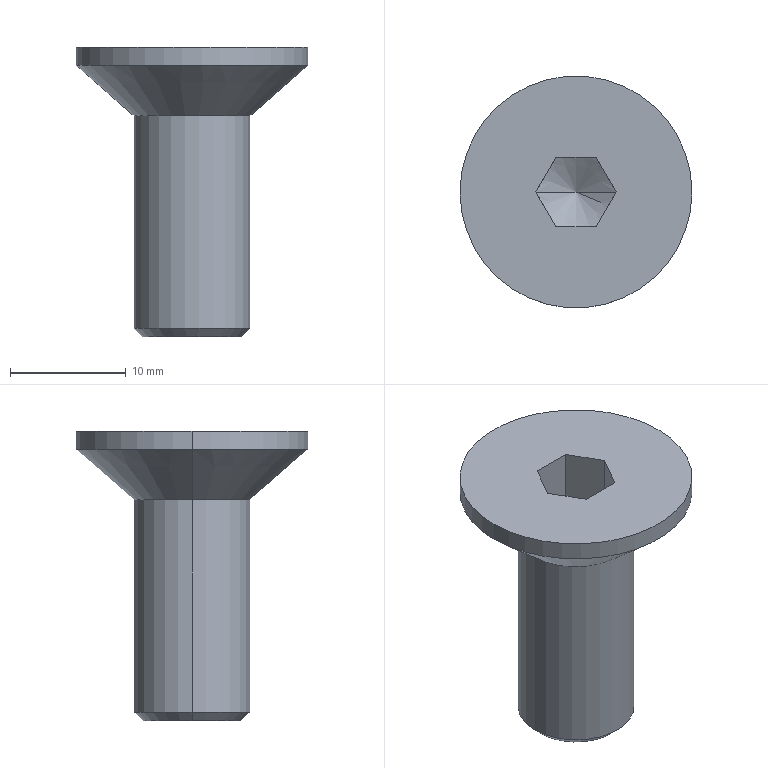Part | Creo | 1 solid | 18 faces | box 20 x 20 x 25 mm | volume 2604 mm3 | plane 8 | cone 6 | cylinder 4 | commonest cylinder face diameters 10 x2 20 x2
STEP:
#1=CARTESIAN_POINT('',(0.,0.,0.));
#2=DIRECTION('',(0.,0.,1.));
#3=DIRECTION('',(1.,0.,0.));
#4=AXIS2_PLACEMENT_3D('',#1,#2,#3);
#5=CARTESIAN_POINT('',(-71.536,0.,310.5));
#6=VERTEX_POINT('',#5);
#7=CARTESIAN_POINT('',(-73.268,3.,310.5));
#8=VERTEX_POINT('',#7);
#9=CARTESIAN_POINT('',(-71.536,0.,310.5));
#10=CARTESIAN_POINT('',(-71.583,0.08105,310.473));
#11=CARTESIAN_POINT('',(-71.675,0.2407,310.423));
#12=CARTESIAN_POINT('',(-71.808,0.471,310.361));
#13=CARTESIAN_POINT('',(-71.939,0.6974,310.311));
#14=CARTESIAN_POINT('',(-72.069,0.9236,310.272));
#15=CARTESIAN_POINT('',(-72.201,1.153,310.245));
#16=CARTESIAN_POINT('',(-72.335,1.384,310.231));
#17=CARTESIAN_POINT('',(-72.469,1.616,310.231));
#18=CARTESIAN_POINT('',(-72.602,1.847,310.245));
#19=CARTESIAN_POINT('',(-72.735,2.076,310.272));
#20=CARTESIAN_POINT('',(-72.865,2.303,310.311));
#21=CARTESIAN_POINT('',(-72.996,2.529,310.361));
#22=CARTESIAN_POINT('',(-73.129,2.759,310.423));
#23=CARTESIAN_POINT('',(-73.221,2.919,310.473));
#24=CARTESIAN_POINT('',(-73.268,3.,310.5));
#25=B_SPLINE_CURVE_WITH_KNOTS('',3,(#9,#10,#11,#12,#13,#14,#15,#16,#17,#18,#19,#20,#21,#22,#23,#24),.UNSPECIFIED.,.F.,.F.,(4,1,1,1,1,1,1,1,1,1,1,1,1,4),(0.,0.07692,0.1538,0.2308,0.3077,0.3846,0.4615,0.5385,0.6154,0.6923,0.7692,0.8462,0.9231,1.),.UNSPECIFIED.);
#26=EDGE_CURVE('',#6,#8,#25,.T.);
#27=ORIENTED_EDGE('',*,*,#26,.F.);
#28=CARTESIAN_POINT('',(-75.,0.,308.5));
#29=VERTEX_POINT('',#28);
#30=CARTESIAN_POINT('',(-75.,0.,308.5));
#31=DIRECTION('',(0.866,0.,0.5));
#32=VECTOR('',#31,4.);
#33=LINE('',#30,#32);
#34=EDGE_CURVE('',#29,#6,#33,.T.);
#35=ORIENTED_EDGE('',*,*,#34,.F.);
#36=CARTESIAN_POINT('',(-78.464,0.,310.5));
#37=VERTEX_POINT('',#36);
#38=CARTESIAN_POINT('',(-75.,0.,308.5));
#39=DIRECTION('',(-0.866,0.,0.5));
#40=VECTOR('',#39,4.);
#41=LINE('',#38,#40);
#42=EDGE_CURVE('',#29,#37,#41,.T.);
#43=ORIENTED_EDGE('',*,*,#42,.T.);
#44=CARTESIAN_POINT('',(-76.732,3.,310.5));
#45=VERTEX_POINT('',#44);
#46=CARTESIAN_POINT('',(-76.732,3.,310.5));
#47=CARTESIAN_POINT('',(-76.779,2.919,310.473));
#48=CARTESIAN_POINT('',(-76.871,2.759,310.423));
#49=CARTESIAN_POINT('',(-77.004,2.529,310.361));
#50=CARTESIAN_POINT('',(-77.135,2.303,310.311));
#51=CARTESIAN_POINT('',(-77.265,2.076,310.272));
#52=CARTESIAN_POINT('',(-77.398,1.847,310.245));
#53=CARTESIAN_POINT('',(-77.531,1.616,310.231));
#54=CARTESIAN_POINT('',(-77.665,1.384,310.231));
#55=CARTESIAN_POINT('',(-77.799,1.153,310.245));
#56=CARTESIAN_POINT('',(-77.931,0.9236,310.272));
#57=CARTESIAN_POINT('',(-78.061,0.6974,310.311));
#58=CARTESIAN_POINT('',(-78.192,0.471,310.361));
#59=CARTESIAN_POINT('',(-78.325,0.2407,310.423));
#60=CARTESIAN_POINT('',(-78.417,0.08105,310.473));
#61=CARTESIAN_POINT('',(-78.464,0.,310.5));
#62=B_SPLINE_CURVE_WITH_KNOTS('',3,(#46,#47,#48,#49,#50,#51,#52,#53,#54,#55,#56,#57,#58,#59,#60,#61),.UNSPECIFIED.,.F.,.F.,(4,1,1,1,1,1,1,1,1,1,1,1,1,4),(0.,0.07692,0.1538,0.2308,0.3077,0.3846,0.4615,0.5385,0.6154,0.6923,0.7692,0.8462,0.9231,1.),.UNSPECIFIED.);
#63=EDGE_CURVE('',#45,#37,#62,.T.);
#64=ORIENTED_EDGE('',*,*,#63,.F.);
#65=CARTESIAN_POINT('',(-73.268,3.,310.5));
#66=CARTESIAN_POINT('',(-73.361,3.,310.473));
#67=CARTESIAN_POINT('',(-73.545,3.,310.423));
#68=CARTESIAN_POINT('',(-73.811,3.,310.361));
#69=CARTESIAN_POINT('',(-74.072,3.,310.311));
#70=CARTESIAN_POINT('',(-74.333,3.,310.272));
#71=CARTESIAN_POINT('',(-74.598,3.,310.245));
#72=CARTESIAN_POINT('',(-74.865,3.,310.231));
#73=CARTESIAN_POINT('',(-75.134,3.,310.231));
#74=CARTESIAN_POINT('',(-75.402,3.,310.245));
#75=CARTESIAN_POINT('',(-75.667,3.,310.272));
#76=CARTESIAN_POINT('',(-75.928,3.,310.311));
#77=CARTESIAN_POINT('',(-76.189,3.,310.361));
#78=CARTESIAN_POINT('',(-76.455,3.,310.423));
#79=CARTESIAN_POINT('',(-76.639,3.,310.473));
#80=CARTESIAN_POINT('',(-76.732,3.,310.5));
#81=B_SPLINE_CURVE_WITH_KNOTS('',3,(#65,#66,#67,#68,#69,#70,#71,#72,#73,#74,#75,#76,#77,#78,#79,#80),.UNSPECIFIED.,.F.,.F.,(4,1,1,1,1,1,1,1,1,1,1,1,1,4),(0.,0.07692,0.1538,0.2308,0.3077,0.3846,0.4615,0.5385,0.6154,0.6923,0.7692,0.8462,0.9231,1.),.UNSPECIFIED.);
#82=EDGE_CURVE('',#8,#45,#81,.T.);
#83=ORIENTED_EDGE('',*,*,#82,.F.);
#84=EDGE_LOOP('',(#27,#35,#43,#64,#83));
#85=FACE_OUTER_BOUND('',#84,.F.);
#86=CARTESIAN_POINT('',(-75.,0.,309.52));
#87=DIRECTION('',(0.,0.,1.));
#88=DIRECTION('',(1.,0.,0.));
#89=AXIS2_PLACEMENT_3D('',#86,#87,#88);
#90=CONICAL_SURFACE('',#89,1.767,60.);
#91=ADVANCED_FACE('',(#85),#90,.F.);
#92=CARTESIAN_POINT('',(-73.268,3.,315.5));
#93=VERTEX_POINT('',#92);
#94=CARTESIAN_POINT('',(-71.536,0.,315.5));
#95=VERTEX_POINT('',#94);
#96=CARTESIAN_POINT('',(-73.268,3.,315.5));
#97=DIRECTION('',(0.5,-0.866,0.));
#98=VECTOR('',#97,3.464);
#99=LINE('',#96,#98);
#100=EDGE_CURVE('',#93,#95,#99,.T.);
#101=ORIENTED_EDGE('',*,*,#100,.T.);
#102=CARTESIAN_POINT('',(-71.536,0.,315.5));
#103=DIRECTION('',(0.,0.,-1.));
#104=VECTOR('',#103,5.);
#105=LINE('',#102,#104);
#106=EDGE_CURVE('',#95,#6,#105,.T.);
#107=ORIENTED_EDGE('',*,*,#106,.T.);
#108=ORIENTED_EDGE('',*,*,#26,.T.);
#109=CARTESIAN_POINT('',(-73.268,3.,315.5));
#110=DIRECTION('',(0.,0.,-1.));
#111=VECTOR('',#110,5.);
#112=LINE('',#109,#111);
#113=EDGE_CURVE('',#93,#8,#112,.T.);
#114=ORIENTED_EDGE('',*,*,#113,.F.);
#115=EDGE_LOOP('',(#101,#107,#108,#114));
#116=FACE_OUTER_BOUND('',#115,.F.);
#117=CARTESIAN_POINT('',(-71.536,0.,310.5));
#118=DIRECTION('',(0.866,0.5,0.));
#119=DIRECTION('',(-0.5,0.866,0.));
#120=AXIS2_PLACEMENT_3D('',#117,#118,#119);
#121=PLANE('',#120);
#122=ADVANCED_FACE('',(#116),#121,.F.);
#123=CARTESIAN_POINT('',(-65.,0.,315.5));
#124=VERTEX_POINT('',#123);
#125=CARTESIAN_POINT('',(-85.,0.,315.5));
#126=VERTEX_POINT('',#125);
#127=CARTESIAN_POINT('',(-75.,0.,315.5));
#128=DIRECTION('',(0.,0.,1.));
#129=DIRECTION('',(1.,0.,0.));
#130=AXIS2_PLACEMENT_3D('',#127,#128,#129);
#131=CIRCLE('',#130,10.);
#132=EDGE_CURVE('',#124,#126,#131,.T.);
#133=ORIENTED_EDGE('',*,*,#132,.F.);
#134=CARTESIAN_POINT('',(-75.,0.,315.5));
#135=DIRECTION('',(0.,0.,1.));
#136=DIRECTION('',(-1.,0.,0.));
#137=AXIS2_PLACEMENT_3D('',#134,#135,#136);
#138=CIRCLE('',#137,10.);
#139=EDGE_CURVE('',#126,#124,#138,.T.);
#140=ORIENTED_EDGE('',*,*,#139,.F.);
#141=EDGE_LOOP('',(#133,#140));
#142=FACE_OUTER_BOUND('',#141,.F.);
#143=CARTESIAN_POINT('',(-76.732,3.,315.5));
#144=VERTEX_POINT('',#143);
#145=CARTESIAN_POINT('',(-76.732,3.,315.5));
#146=DIRECTION('',(1.,0.,0.));
#147=VECTOR('',#146,3.464);
#148=LINE('',#145,#147);
#149=EDGE_CURVE('',#144,#93,#148,.T.);
#150=ORIENTED_EDGE('',*,*,#149,.F.);
#151=CARTESIAN_POINT('',(-78.464,0.,315.5));
#152=VERTEX_POINT('',#151);
#153=CARTESIAN_POINT('',(-78.464,0.,315.5));
#154=DIRECTION('',(0.5,0.866,0.));
#155=VECTOR('',#154,3.464);
#156=LINE('',#153,#155);
#157=EDGE_CURVE('',#152,#144,#156,.T.);
#158=ORIENTED_EDGE('',*,*,#157,.F.);
#159=CARTESIAN_POINT('',(-76.732,-3.,315.5));
#160=VERTEX_POINT('',#159);
#161=CARTESIAN_POINT('',(-76.732,-3.,315.5));
#162=DIRECTION('',(-0.5,0.866,0.));
#163=VECTOR('',#162,3.464);
#164=LINE('',#161,#163);
#165=EDGE_CURVE('',#160,#152,#164,.T.);
#166=ORIENTED_EDGE('',*,*,#165,.F.);
#167=CARTESIAN_POINT('',(-73.268,-3.,315.5));
#168=VERTEX_POINT('',#167);
#169=CARTESIAN_POINT('',(-73.268,-3.,315.5));
#170=DIRECTION('',(-1.,0.,0.));
#171=VECTOR('',#170,3.464);
#172=LINE('',#169,#171);
#173=EDGE_CURVE('',#168,#160,#172,.T.);
#174=ORIENTED_EDGE('',*,*,#173,.F.);
#175=CARTESIAN_POINT('',(-71.536,0.,315.5));
#176=DIRECTION('',(-0.5,-0.866,0.));
#177=VECTOR('',#176,3.464);
#178=LINE('',#175,#177);
#179=EDGE_CURVE('',#95,#168,#178,.T.);
#180=ORIENTED_EDGE('',*,*,#179,.F.);
#181=ORIENTED_EDGE('',*,*,#100,.F.);
#182=EDGE_LOOP('',(#150,#158,#166,#174,#180,#181));
#183=FACE_BOUND('',#182,.F.);
#184=CARTESIAN_POINT('',(-65.,0.,315.5));
#185=DIRECTION('',(0.,0.,-1.));
#186=DIRECTION('',(-1.,0.,0.));
#187=AXIS2_PLACEMENT_3D('',#184,#185,#186);
#188=PLANE('',#187);
#189=ADVANCED_FACE('',(#142,#183),#188,.F.);
#190=ORIENTED_EDGE('',*,*,#149,.T.);
#191=ORIENTED_EDGE('',*,*,#113,.T.);
#192=ORIENTED_EDGE('',*,*,#82,.T.);
#193=CARTESIAN_POINT('',(-76.732,3.,315.5));
#194=DIRECTION('',(0.,0.,-1.));
#195=VECTOR('',#194,5.);
#196=LINE('',#193,#195);
#197=EDGE_CURVE('',#144,#45,#196,.T.);
#198=ORIENTED_EDGE('',*,*,#197,.F.);
#199=EDGE_LOOP('',(#190,#191,#192,#198));
#200=FACE_OUTER_BOUND('',#199,.F.);
#201=CARTESIAN_POINT('',(-73.268,3.,310.5));
#202=DIRECTION('',(0.,1.,0.));
#203=DIRECTION('',(0.,0.,1.));
#204=AXIS2_PLACEMENT_3D('',#201,#202,#203);
#205=PLANE('',#204);
#206=ADVANCED_FACE('',(#200),#205,.F.);
#207=ORIENTED_EDGE('',*,*,#157,.T.);
#208=ORIENTED_EDGE('',*,*,#197,.T.);
#209=ORIENTED_EDGE('',*,*,#63,.T.);
#210=CARTESIAN_POINT('',(-78.464,0.,315.5));
#211=DIRECTION('',(0.,0.,-1.));
#212=VECTOR('',#211,5.);
#213=LINE('',#210,#212);
#214=EDGE_CURVE('',#152,#37,#213,.T.);
#215=ORIENTED_EDGE('',*,*,#214,.F.);
#216=EDGE_LOOP('',(#207,#208,#209,#215));
#217=FACE_OUTER_BOUND('',#216,.F.);
#218=CARTESIAN_POINT('',(-76.732,3.,310.5));
#219=DIRECTION('',(-0.866,0.5,0.));
#220=DIRECTION('',(-0.5,-0.866,0.));
#221=AXIS2_PLACEMENT_3D('',#218,#219,#220);
#222=PLANE('',#221);
#223=ADVANCED_FACE('',(#217),#222,.F.);
#224=ORIENTED_EDGE('',*,*,#165,.T.);
#225=ORIENTED_EDGE('',*,*,#214,.T.);
#226=CARTESIAN_POINT('',(-76.732,-3.,310.5));
#227=VERTEX_POINT('',#226);
#228=CARTESIAN_POINT('',(-78.464,0.,310.5));
#229=CARTESIAN_POINT('',(-78.417,-0.08105,310.473));
#230=CARTESIAN_POINT('',(-78.325,-0.2407,310.423));
#231=CARTESIAN_POINT('',(-78.192,-0.471,310.361));
#232=CARTESIAN_POINT('',(-78.061,-0.6974,310.311));
#233=CARTESIAN_POINT('',(-77.931,-0.9236,310.272));
#234=CARTESIAN_POINT('',(-77.799,-1.153,310.245));
#235=CARTESIAN_POINT('',(-77.665,-1.384,310.231));
#236=CARTESIAN_POINT('',(-77.531,-1.616,310.231));
#237=CARTESIAN_POINT('',(-77.398,-1.847,310.245));
#238=CARTESIAN_POINT('',(-77.265,-2.076,310.272));
#239=CARTESIAN_POINT('',(-77.135,-2.303,310.311));
#240=CARTESIAN_POINT('',(-77.004,-2.529,310.361));
#241=CARTESIAN_POINT('',(-76.871,-2.759,310.423));
#242=CARTESIAN_POINT('',(-76.779,-2.919,310.473));
#243=CARTESIAN_POINT('',(-76.732,-3.,310.5));
#244=B_SPLINE_CURVE_WITH_KNOTS('',3,(#228,#229,#230,#231,#232,#233,#234,#235,#236,#237,#238,#239,#240,#241,#242,#243),.UNSPECIFIED.,.F.,.F.,(4,1,1,1,1,1,1,1,1,1,1,1,1,4),(0.,0.07692,0.1538,0.2308,0.3077,0.3846,0.4615,0.5385,0.6154,0.6923,0.7692,0.8462,0.9231,1.),.UNSPECIFIED.);
#245=EDGE_CURVE('',#37,#227,#244,.T.);
#246=ORIENTED_EDGE('',*,*,#245,.T.);
#247=CARTESIAN_POINT('',(-76.732,-3.,315.5));
#248=DIRECTION('',(0.,0.,-1.));
#249=VECTOR('',#248,5.);
#250=LINE('',#247,#249);
#251=EDGE_CURVE('',#160,#227,#250,.T.);
#252=ORIENTED_EDGE('',*,*,#251,.F.);
#253=EDGE_LOOP('',(#224,#225,#246,#252));
#254=FACE_OUTER_BOUND('',#253,.F.);
#255=CARTESIAN_POINT('',(-78.464,0.,310.5));
#256=DIRECTION('',(-0.866,-0.5,0.));
#257=DIRECTION('',(0.5,-0.866,0.));
#258=AXIS2_PLACEMENT_3D('',#255,#256,#257);
#259=PLANE('',#258);
#260=ADVANCED_FACE('',(#254),#259,.F.);
#261=CARTESIAN_POINT('',(-73.268,-3.,310.5));
#262=VERTEX_POINT('',#261);
#263=CARTESIAN_POINT('',(-76.732,-3.,310.5));
#264=CARTESIAN_POINT('',(-76.639,-3.,310.473));
#265=CARTESIAN_POINT('',(-76.455,-3.,310.423));
#266=CARTESIAN_POINT('',(-76.189,-3.,310.361));
#267=CARTESIAN_POINT('',(-75.928,-3.,310.311));
#268=CARTESIAN_POINT('',(-75.667,-3.,310.272));
#269=CARTESIAN_POINT('',(-75.402,-3.,310.245));
#270=CARTESIAN_POINT('',(-75.134,-3.,310.231));
#271=CARTESIAN_POINT('',(-74.865,-3.,310.231));
#272=CARTESIAN_POINT('',(-74.598,-3.,310.245));
#273=CARTESIAN_POINT('',(-74.333,-3.,310.272));
#274=CARTESIAN_POINT('',(-74.072,-3.,310.311));
#275=CARTESIAN_POINT('',(-73.811,-3.,310.361));
#276=CARTESIAN_POINT('',(-73.545,-3.,310.423));
#277=CARTESIAN_POINT('',(-73.361,-3.,310.473));
#278=CARTESIAN_POINT('',(-73.268,-3.,310.5));
#279=B_SPLINE_CURVE_WITH_KNOTS('',3,(#263,#264,#265,#266,#267,#268,#269,#270,#271,#272,#273,#274,#275,#276,#277,#278),.UNSPECIFIED.,.F.,.F.,(4,1,1,1,1,1,1,1,1,1,1,1,1,4),(0.,0.07692,0.1538,0.2308,0.3077,0.3846,0.4615,0.5385,0.6154,0.6923,0.7692,0.8462,0.9231,1.),.UNSPECIFIED.);
#280=EDGE_CURVE('',#227,#262,#279,.T.);
#281=ORIENTED_EDGE('',*,*,#280,.F.);
#282=ORIENTED_EDGE('',*,*,#245,.F.);
#283=ORIENTED_EDGE('',*,*,#42,.F.);
#284=ORIENTED_EDGE('',*,*,#34,.T.);
#285=CARTESIAN_POINT('',(-73.268,-3.,310.5));
#286=CARTESIAN_POINT('',(-73.221,-2.919,310.473));
#287=CARTESIAN_POINT('',(-73.129,-2.759,310.423));
#288=CARTESIAN_POINT('',(-72.996,-2.529,310.361));
#289=CARTESIAN_POINT('',(-72.865,-2.303,310.311));
#290=CARTESIAN_POINT('',(-72.735,-2.076,310.272));
#291=CARTESIAN_POINT('',(-72.602,-1.847,310.245));
#292=CARTESIAN_POINT('',(-72.469,-1.616,310.231));
#293=CARTESIAN_POINT('',(-72.335,-1.384,310.231));
#294=CARTESIAN_POINT('',(-72.201,-1.153,310.245));
#295=CARTESIAN_POINT('',(-72.069,-0.9236,310.272));
#296=CARTESIAN_POINT('',(-71.939,-0.6974,310.311));
#297=CARTESIAN_POINT('',(-71.808,-0.471,310.361));
#298=CARTESIAN_POINT('',(-71.675,-0.2407,310.423));
#299=CARTESIAN_POINT('',(-71.583,-0.08105,310.473));
#300=CARTESIAN_POINT('',(-71.536,0.,310.5));
#301=B_SPLINE_CURVE_WITH_KNOTS('',3,(#285,#286,#287,#288,#289,#290,#291,#292,#293,#294,#295,#296,#297,#298,#299,#300),.UNSPECIFIED.,.F.,.F.,(4,1,1,1,1,1,1,1,1,1,1,1,1,4),(0.,0.07692,0.1538,0.2308,0.3077,0.3846,0.4615,0.5385,0.6154,0.6923,0.7692,0.8462,0.9231,1.),.UNSPECIFIED.);
#302=EDGE_CURVE('',#262,#6,#301,.T.);
#303=ORIENTED_EDGE('',*,*,#302,.F.);
#304=EDGE_LOOP('',(#281,#282,#283,#284,#303));
#305=FACE_OUTER_BOUND('',#304,.F.);
#306=CARTESIAN_POINT('',(-75.,0.,309.52));
#307=DIRECTION('',(0.,0.,1.));
#308=DIRECTION('',(1.,0.,0.));
#309=AXIS2_PLACEMENT_3D('',#306,#307,#308);
#310=CONICAL_SURFACE('',#309,1.767,60.);
#311=ADVANCED_FACE('',(#305),#310,.F.);
#312=ORIENTED_EDGE('',*,*,#173,.T.);
#313=ORIENTED_EDGE('',*,*,#251,.T.);
#314=ORIENTED_EDGE('',*,*,#280,.T.);
#315=CARTESIAN_POINT('',(-73.268,-3.,315.5));
#316=DIRECTION('',(0.,0.,-1.));
#317=VECTOR('',#316,5.);
#318=LINE('',#315,#317);
#319=EDGE_CURVE('',#168,#262,#318,.T.);
#320=ORIENTED_EDGE('',*,*,#319,.F.);
#321=EDGE_LOOP('',(#312,#313,#314,#320));
#322=FACE_OUTER_BOUND('',#321,.F.);
#323=CARTESIAN_POINT('',(-76.732,-3.,310.5));
#324=DIRECTION('',(0.,-1.,0.));
#325=DIRECTION('',(0.,0.,-1.));
#326=AXIS2_PLACEMENT_3D('',#323,#324,#325);
#327=PLANE('',#326);
#328=ADVANCED_FACE('',(#322),#327,.F.);
#329=ORIENTED_EDGE('',*,*,#179,.T.);
#330=ORIENTED_EDGE('',*,*,#319,.T.);
#331=ORIENTED_EDGE('',*,*,#302,.T.);
#332=ORIENTED_EDGE('',*,*,#106,.F.);
#333=EDGE_LOOP('',(#329,#330,#331,#332));
#334=FACE_OUTER_BOUND('',#333,.F.);
#335=CARTESIAN_POINT('',(-73.268,-3.,310.5));
#336=DIRECTION('',(0.866,-0.5,0.));
#337=DIRECTION('',(0.5,0.866,0.));
#338=AXIS2_PLACEMENT_3D('',#335,#336,#337);
#339=PLANE('',#338);
#340=ADVANCED_FACE('',(#334),#339,.F.);
#341=ORIENTED_EDGE('',*,*,#132,.T.);
#342=CARTESIAN_POINT('',(-85.,0.,313.913));
#343=VERTEX_POINT('',#342);
#344=CARTESIAN_POINT('',(-85.,0.,313.913));
#345=DIRECTION('',(0.,0.,1.));
#346=VECTOR('',#345,1.587);
#347=LINE('',#344,#346);
#348=EDGE_CURVE('',#343,#126,#347,.T.);
#349=ORIENTED_EDGE('',*,*,#348,.F.);
#350=CARTESIAN_POINT('',(-65.,0.,313.913));
#351=VERTEX_POINT('',#350);
#352=CARTESIAN_POINT('',(-75.,0.,313.913));
#353=DIRECTION('',(0.,0.,-1.));
#354=DIRECTION('',(-1.,0.,0.));
#355=AXIS2_PLACEMENT_3D('',#352,#353,#354);
#356=CIRCLE('',#355,10.);
#357=EDGE_CURVE('',#343,#351,#356,.T.);
#358=ORIENTED_EDGE('',*,*,#357,.T.);
#359=CARTESIAN_POINT('',(-65.,0.,313.913));
#360=DIRECTION('',(0.,0.,1.));
#361=VECTOR('',#360,1.587);
#362=LINE('',#359,#361);
#363=EDGE_CURVE('',#351,#124,#362,.T.);
#364=ORIENTED_EDGE('',*,*,#363,.T.);
#365=EDGE_LOOP('',(#341,#349,#358,#364));
#366=FACE_OUTER_BOUND('',#365,.F.);
#367=CARTESIAN_POINT('',(-75.,0.,316.5));
#368=DIRECTION('',(0.,0.,1.));
#369=DIRECTION('',(1.,0.,0.));
#370=AXIS2_PLACEMENT_3D('',#367,#368,#369);
#371=CYLINDRICAL_SURFACE('',#370,10.);
#372=ADVANCED_FACE('',(#366),#371,.T.);
#373=ORIENTED_EDGE('',*,*,#139,.T.);
#374=ORIENTED_EDGE('',*,*,#363,.F.);
#375=CARTESIAN_POINT('',(-75.,0.,313.913));
#376=DIRECTION('',(0.,0.,-1.));
#377=DIRECTION('',(1.,0.,0.));
#378=AXIS2_PLACEMENT_3D('',#375,#376,#377);
#379=CIRCLE('',#378,10.);
#380=EDGE_CURVE('',#351,#343,#379,.T.);
#381=ORIENTED_EDGE('',*,*,#380,.T.);
#382=ORIENTED_EDGE('',*,*,#348,.T.);
#383=EDGE_LOOP('',(#373,#374,#381,#382));
#384=FACE_OUTER_BOUND('',#383,.F.);
#385=CARTESIAN_POINT('',(-75.,0.,316.5));
#386=DIRECTION('',(0.,0.,1.));
#387=DIRECTION('',(1.,0.,0.));
#388=AXIS2_PLACEMENT_3D('',#385,#386,#387);
#389=CYLINDRICAL_SURFACE('',#388,10.);
#390=ADVANCED_FACE('',(#384),#389,.T.);
#391=CARTESIAN_POINT('',(-80.,0.,309.565));
#392=VERTEX_POINT('',#391);
#393=CARTESIAN_POINT('',(-70.,0.,309.565));
#394=VERTEX_POINT('',#393);
#395=CARTESIAN_POINT('',(-75.,0.,309.565));
#396=DIRECTION('',(0.,0.,1.));
#397=DIRECTION('',(-1.,0.,0.));
#398=AXIS2_PLACEMENT_3D('',#395,#396,#397);
#399=CIRCLE('',#398,5.);
#400=EDGE_CURVE('',#392,#394,#399,.T.);
#401=ORIENTED_EDGE('',*,*,#400,.F.);
#402=CARTESIAN_POINT('',(-80.,0.,309.565));
#403=DIRECTION('',(-0.7546,0.,0.6562));
#404=VECTOR('',#403,6.626);
#405=LINE('',#402,#404);
#406=EDGE_CURVE('',#392,#343,#405,.T.);
#407=ORIENTED_EDGE('',*,*,#406,.T.);
#408=ORIENTED_EDGE('',*,*,#380,.F.);
#409=CARTESIAN_POINT('',(-70.,0.,309.565));
#410=DIRECTION('',(0.7546,0.,0.6562));
#411=VECTOR('',#410,6.626);
#412=LINE('',#409,#411);
#413=EDGE_CURVE('',#394,#351,#412,.T.);
#414=ORIENTED_EDGE('',*,*,#413,.F.);
#415=EDGE_LOOP('',(#401,#407,#408,#414));
#416=FACE_OUTER_BOUND('',#415,.F.);
#417=CARTESIAN_POINT('',(-75.,0.,311.739));
#418=DIRECTION('',(0.,0.,1.));
#419=DIRECTION('',(1.,0.,0.));
#420=AXIS2_PLACEMENT_3D('',#417,#418,#419);
#421=CONICAL_SURFACE('',#420,7.5,48.991);
#422=ADVANCED_FACE('',(#416),#421,.T.);
#423=ORIENTED_EDGE('',*,*,#400,.T.);
#424=CARTESIAN_POINT('',(-70.,0.,291.25));
#425=VERTEX_POINT('',#424);
#426=CARTESIAN_POINT('',(-70.,0.,291.25));
#427=DIRECTION('',(0.,0.,1.));
#428=VECTOR('',#427,18.315);
#429=LINE('',#426,#428);
#430=EDGE_CURVE('',#425,#394,#429,.T.);
#431=ORIENTED_EDGE('',*,*,#430,.F.);
#432=CARTESIAN_POINT('',(-80.,0.,291.25));
#433=VERTEX_POINT('',#432);
#434=CARTESIAN_POINT('',(-75.,0.,291.25));
#435=DIRECTION('',(0.,0.,-1.));
#436=DIRECTION('',(1.,0.,0.));
#437=AXIS2_PLACEMENT_3D('',#434,#435,#436);
#438=CIRCLE('',#437,5.);
#439=EDGE_CURVE('',#425,#433,#438,.T.);
#440=ORIENTED_EDGE('',*,*,#439,.T.);
#441=CARTESIAN_POINT('',(-80.,0.,291.25));
#442=DIRECTION('',(0.,0.,1.));
#443=VECTOR('',#442,18.315);
#444=LINE('',#441,#443);
#445=EDGE_CURVE('',#433,#392,#444,.T.);
#446=ORIENTED_EDGE('',*,*,#445,.T.);
#447=EDGE_LOOP('',(#423,#431,#440,#446));
#448=FACE_OUTER_BOUND('',#447,.F.);
#449=CARTESIAN_POINT('',(-75.,0.,316.5));
#450=DIRECTION('',(0.,0.,1.));
#451=DIRECTION('',(1.,0.,0.));
#452=AXIS2_PLACEMENT_3D('',#449,#450,#451);
#453=CYLINDRICAL_SURFACE('',#452,5.);
#454=ADVANCED_FACE('',(#448),#453,.T.);
#455=CARTESIAN_POINT('',(-75.,0.,309.565));
#456=DIRECTION('',(0.,0.,1.));
#457=DIRECTION('',(1.,0.,0.));
#458=AXIS2_PLACEMENT_3D('',#455,#456,#457);
#459=CIRCLE('',#458,5.);
#460=EDGE_CURVE('',#394,#392,#459,.T.);
#461=ORIENTED_EDGE('',*,*,#460,.T.);
#462=ORIENTED_EDGE('',*,*,#445,.F.);
#463=CARTESIAN_POINT('',(-75.,0.,291.25));
#464=DIRECTION('',(0.,0.,-1.));
#465=DIRECTION('',(-1.,0.,0.));
#466=AXIS2_PLACEMENT_3D('',#463,#464,#465);
#467=CIRCLE('',#466,5.);
#468=EDGE_CURVE('',#433,#425,#467,.T.);
#469=ORIENTED_EDGE('',*,*,#468,.T.);
#470=ORIENTED_EDGE('',*,*,#430,.T.);
#471=EDGE_LOOP('',(#461,#462,#469,#470));
#472=FACE_OUTER_BOUND('',#471,.F.);
#473=CARTESIAN_POINT('',(-75.,0.,316.5));
#474=DIRECTION('',(0.,0.,1.));
#475=DIRECTION('',(1.,0.,0.));
#476=AXIS2_PLACEMENT_3D('',#473,#474,#475);
#477=CYLINDRICAL_SURFACE('',#476,5.);
#478=ADVANCED_FACE('',(#472),#477,.T.);
#479=ORIENTED_EDGE('',*,*,#460,.F.);
#480=ORIENTED_EDGE('',*,*,#413,.T.);
#481=ORIENTED_EDGE('',*,*,#357,.F.);
#482=ORIENTED_EDGE('',*,*,#406,.F.);
#483=EDGE_LOOP('',(#479,#480,#481,#482));
#484=FACE_OUTER_BOUND('',#483,.F.);
#485=CARTESIAN_POINT('',(-75.,0.,311.739));
#486=DIRECTION('',(0.,0.,1.));
#487=DIRECTION('',(1.,0.,0.));
#488=AXIS2_PLACEMENT_3D('',#485,#486,#487);
#489=CONICAL_SURFACE('',#488,7.5,48.991);
#490=ADVANCED_FACE('',(#484),#489,.T.);
#491=ORIENTED_EDGE('',*,*,#468,.F.);
#492=CARTESIAN_POINT('',(-79.25,0.,290.5));
#493=VERTEX_POINT('',#492);
#494=CARTESIAN_POINT('',(-79.25,0.,290.5));
#495=DIRECTION('',(-0.7071,0.,0.7071));
#496=VECTOR('',#495,1.061);
#497=LINE('',#494,#496);
#498=EDGE_CURVE('',#493,#433,#497,.T.);
#499=ORIENTED_EDGE('',*,*,#498,.F.);
#500=CARTESIAN_POINT('',(-70.75,0.,290.5));
#501=VERTEX_POINT('',#500);
#502=CARTESIAN_POINT('',(-75.,0.,290.5));
#503=DIRECTION('',(0.,0.,-1.));
#504=DIRECTION('',(-1.,0.,0.));
#505=AXIS2_PLACEMENT_3D('',#502,#503,#504);
#506=CIRCLE('',#505,4.25);
#507=EDGE_CURVE('',#493,#501,#506,.T.);
#508=ORIENTED_EDGE('',*,*,#507,.T.);
#509=CARTESIAN_POINT('',(-70.75,0.,290.5));
#510=DIRECTION('',(0.7071,0.,0.7071));
#511=VECTOR('',#510,1.061);
#512=LINE('',#509,#511);
#513=EDGE_CURVE('',#501,#425,#512,.T.);
#514=ORIENTED_EDGE('',*,*,#513,.T.);
#515=EDGE_LOOP('',(#491,#499,#508,#514));
#516=FACE_OUTER_BOUND('',#515,.F.);
#517=CARTESIAN_POINT('',(-75.,0.,290.875));
#518=DIRECTION('',(0.,0.,1.));
#519=DIRECTION('',(1.,0.,0.));
#520=AXIS2_PLACEMENT_3D('',#517,#518,#519);
#521=CONICAL_SURFACE('',#520,4.625,45.);
#522=ADVANCED_FACE('',(#516),#521,.T.);
#523=ORIENTED_EDGE('',*,*,#439,.F.);
#524=ORIENTED_EDGE('',*,*,#513,.F.);
#525=CARTESIAN_POINT('',(-75.,0.,290.5));
#526=DIRECTION('',(0.,0.,-1.));
#527=DIRECTION('',(1.,0.,0.));
#528=AXIS2_PLACEMENT_3D('',#525,#526,#527);
#529=CIRCLE('',#528,4.25);
#530=EDGE_CURVE('',#501,#493,#529,.T.);
#531=ORIENTED_EDGE('',*,*,#530,.T.);
#532=ORIENTED_EDGE('',*,*,#498,.T.);
#533=EDGE_LOOP('',(#523,#524,#531,#532));
#534=FACE_OUTER_BOUND('',#533,.F.);
#535=CARTESIAN_POINT('',(-75.,0.,290.875));
#536=DIRECTION('',(0.,0.,1.));
#537=DIRECTION('',(1.,0.,0.));
#538=AXIS2_PLACEMENT_3D('',#535,#536,#537);
#539=CONICAL_SURFACE('',#538,4.625,45.);
#540=ADVANCED_FACE('',(#534),#539,.T.);
#541=ORIENTED_EDGE('',*,*,#530,.F.);
#542=ORIENTED_EDGE('',*,*,#507,.F.);
#543=EDGE_LOOP('',(#541,#542));
#544=FACE_OUTER_BOUND('',#543,.F.);
#545=CARTESIAN_POINT('',(-75.,0.,290.5));
#546=DIRECTION('',(0.,0.,1.));
#547=DIRECTION('',(1.,0.,0.));
#548=AXIS2_PLACEMENT_3D('',#545,#546,#547);
#549=PLANE('',#548);
#550=ADVANCED_FACE('',(#544),#549,.F.);
#551=CLOSED_SHELL('',(#91,#122,#189,#206,#223,#260,#311,#328,#340,#372,#390,#422,#454,#478,#490,#522,#540,#550));
#552=MANIFOLD_SOLID_BREP('',#551);
#553=(LENGTH_UNIT()NAMED_UNIT(*)SI_UNIT(.MILLI.,.METRE.));
#554=UNCERTAINTY_MEASURE_WITH_UNIT(LENGTH_MEASURE(0.003775),#553,'','');
#555=(NAMED_UNIT(*)PLANE_ANGLE_UNIT()SI_UNIT($,.RADIAN.));
#556=PLANE_ANGLE_MEASURE_WITH_UNIT(PLANE_ANGLE_MEASURE(0.01745),#555);
#557=(CONVERSION_BASED_UNIT('DEGREE',#556)NAMED_UNIT(*)PLANE_ANGLE_UNIT());
#558=(NAMED_UNIT(*)SI_UNIT($,.STERADIAN.)SOLID_ANGLE_UNIT());
#559=(GEOMETRIC_REPRESENTATION_CONTEXT(3)GLOBAL_UNCERTAINTY_ASSIGNED_CONTEXT((#554))GLOBAL_UNIT_ASSIGNED_CONTEXT((#553,#557,#558))REPRESENTATION_CONTEXT('',''));
#560=ADVANCED_BREP_SHAPE_REPRESENTATION('',(#4,#552),#559);